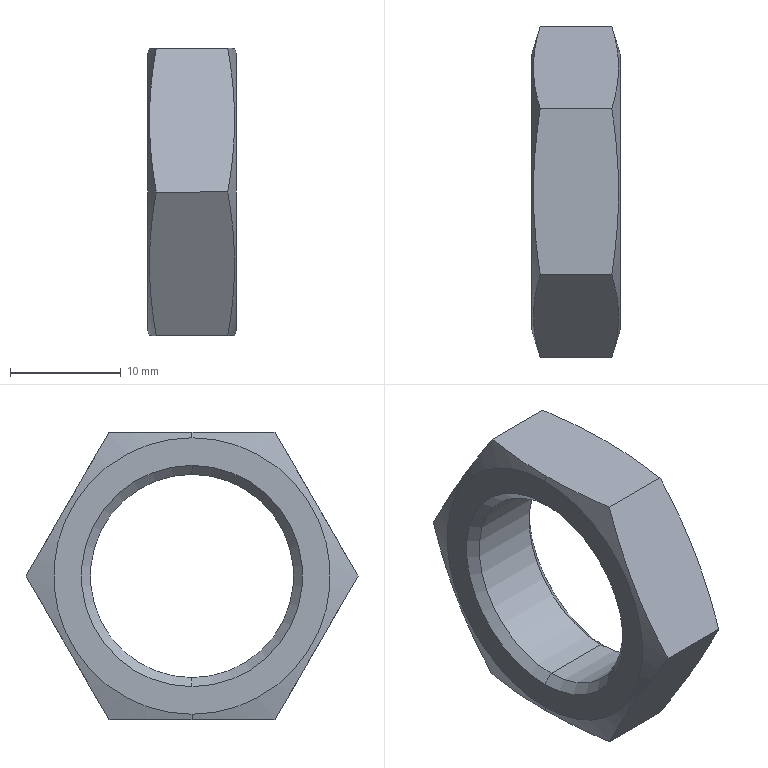Part | SolidWorks | features BaseBody 1 | 1 solid | 18 faces | box 8 x 30.022 x 26 mm | volume 2480 mm3 | cone 8 | plane 8 | cylinder 2 | commonest cylinder face diameters 18.376 x2
STEP:
#1=CARTESIAN_POINT('',(0.812,0.,9.188));
#2=VERTEX_POINT('',#1);
#3=CARTESIAN_POINT('',(0.812,0.,-9.188));
#4=VERTEX_POINT('',#3);
#5=CARTESIAN_POINT('',(0.812,0.,0.));
#6=DIRECTION('',(1.,0.,0.));
#7=DIRECTION('',(0.,0.,-1.));
#8=AXIS2_PLACEMENT_3D('',#5,#6,#7);
#9=CIRCLE('',#8,9.188);
#10=EDGE_CURVE('',#2,#4,#9,.T.);
#11=ORIENTED_EDGE('',*,*,#10,.F.);
#12=CARTESIAN_POINT('',(7.188,0.,9.188));
#13=VERTEX_POINT('',#12);
#14=CARTESIAN_POINT('',(0.,0.,9.188));
#15=DIRECTION('',(1.,0.,0.));
#16=VECTOR('',#15,1000.);
#17=LINE('',#14,#16);
#18=EDGE_CURVE('',#2,#13,#17,.T.);
#19=ORIENTED_EDGE('',*,*,#18,.T.);
#20=CARTESIAN_POINT('',(7.188,0.,-9.188));
#21=VERTEX_POINT('',#20);
#22=CARTESIAN_POINT('',(7.188,0.,0.));
#23=DIRECTION('',(-1.,0.,0.));
#24=DIRECTION('',(0.,0.,-1.));
#25=AXIS2_PLACEMENT_3D('',#22,#23,#24);
#26=CIRCLE('',#25,9.188);
#27=EDGE_CURVE('',#21,#13,#26,.T.);
#28=ORIENTED_EDGE('',*,*,#27,.F.);
#29=CARTESIAN_POINT('',(0.,0.,-9.188));
#30=DIRECTION('',(1.,0.,0.));
#31=VECTOR('',#30,1000.);
#32=LINE('',#29,#31);
#33=EDGE_CURVE('',#4,#21,#32,.T.);
#34=ORIENTED_EDGE('',*,*,#33,.F.);
#35=EDGE_LOOP('',(#11,#19,#28,#34));
#36=FACE_OUTER_BOUND('',#35,.T.);
#37=CARTESIAN_POINT('',(0.,0.,0.));
#38=DIRECTION('',(1.,0.,0.));
#39=DIRECTION('',(0.,0.,-1.));
#40=AXIS2_PLACEMENT_3D('',#37,#38,#39);
#41=CYLINDRICAL_SURFACE('',#40,9.188);
#42=ADVANCED_FACE('',(#36),#41,.F.);
#43=ORIENTED_EDGE('',*,*,#27,.T.);
#44=CARTESIAN_POINT('',(8.,0.,10.));
#45=VERTEX_POINT('',#44);
#46=CARTESIAN_POINT('',(8.,0.,10.));
#47=DIRECTION('',(0.7071,0.,0.7071));
#48=VECTOR('',#47,1000.);
#49=LINE('',#46,#48);
#50=EDGE_CURVE('',#13,#45,#49,.T.);
#51=ORIENTED_EDGE('',*,*,#50,.T.);
#52=CARTESIAN_POINT('',(8.,0.,-10.));
#53=VERTEX_POINT('',#52);
#54=CARTESIAN_POINT('',(8.,0.,0.));
#55=DIRECTION('',(-1.,0.,0.));
#56=DIRECTION('',(0.,0.,-1.));
#57=AXIS2_PLACEMENT_3D('',#54,#55,#56);
#58=CIRCLE('',#57,10.);
#59=EDGE_CURVE('',#53,#45,#58,.T.);
#60=ORIENTED_EDGE('',*,*,#59,.F.);
#61=CARTESIAN_POINT('',(8.,0.,-10.));
#62=DIRECTION('',(0.7071,0.,-0.7071));
#63=VECTOR('',#62,1000.);
#64=LINE('',#61,#63);
#65=EDGE_CURVE('',#21,#53,#64,.T.);
#66=ORIENTED_EDGE('',*,*,#65,.F.);
#67=EDGE_LOOP('',(#43,#51,#60,#66));
#68=FACE_OUTER_BOUND('',#67,.T.);
#69=CARTESIAN_POINT('',(8.,0.,0.));
#70=DIRECTION('',(1.,0.,0.));
#71=DIRECTION('',(0.,0.,-1.));
#72=AXIS2_PLACEMENT_3D('',#69,#70,#71);
#73=CONICAL_SURFACE('',#72,10.,0.7854);
#74=ADVANCED_FACE('',(#68),#73,.F.);
#75=ORIENTED_EDGE('',*,*,#10,.T.);
#76=CARTESIAN_POINT('',(0.,0.,-10.));
#77=VERTEX_POINT('',#76);
#78=CARTESIAN_POINT('',(0.,0.,-10.));
#79=DIRECTION('',(-0.7071,0.,-0.7071));
#80=VECTOR('',#79,1000.);
#81=LINE('',#78,#80);
#82=EDGE_CURVE('',#4,#77,#81,.T.);
#83=ORIENTED_EDGE('',*,*,#82,.T.);
#84=CARTESIAN_POINT('',(0.,0.,10.));
#85=VERTEX_POINT('',#84);
#86=CARTESIAN_POINT('',(0.,0.,0.));
#87=DIRECTION('',(1.,0.,0.));
#88=DIRECTION('',(0.,0.,1.));
#89=AXIS2_PLACEMENT_3D('',#86,#87,#88);
#90=CIRCLE('',#89,10.);
#91=EDGE_CURVE('',#85,#77,#90,.T.);
#92=ORIENTED_EDGE('',*,*,#91,.F.);
#93=CARTESIAN_POINT('',(0.,0.,10.));
#94=DIRECTION('',(-0.7071,0.,0.7071));
#95=VECTOR('',#94,1000.);
#96=LINE('',#93,#95);
#97=EDGE_CURVE('',#2,#85,#96,.T.);
#98=ORIENTED_EDGE('',*,*,#97,.F.);
#99=EDGE_LOOP('',(#75,#83,#92,#98));
#100=FACE_OUTER_BOUND('',#99,.T.);
#101=CARTESIAN_POINT('',(0.,0.,0.));
#102=DIRECTION('',(-1.,0.,0.));
#103=DIRECTION('',(0.,0.,1.));
#104=AXIS2_PLACEMENT_3D('',#101,#102,#103);
#105=CONICAL_SURFACE('',#104,10.,0.7854);
#106=ADVANCED_FACE('',(#100),#105,.F.);
#107=CARTESIAN_POINT('',(8.,0.,-12.5));
#108=VERTEX_POINT('',#107);
#109=CARTESIAN_POINT('',(8.,0.,12.5));
#110=VERTEX_POINT('',#109);
#111=CARTESIAN_POINT('',(8.,0.,0.));
#112=DIRECTION('',(1.,0.,0.));
#113=DIRECTION('',(0.,0.,1.));
#114=AXIS2_PLACEMENT_3D('',#111,#112,#113);
#115=CIRCLE('',#114,12.5);
#116=EDGE_CURVE('',#108,#110,#115,.T.);
#117=ORIENTED_EDGE('',*,*,#116,.F.);
#118=CARTESIAN_POINT('',(7.848,0.,-13.));
#119=VERTEX_POINT('',#118);
#120=CARTESIAN_POINT('',(7.231,0.,-15.026));
#121=DIRECTION('',(-0.2912,0.,-0.9567));
#122=VECTOR('',#121,1000.);
#123=LINE('',#120,#122);
#124=EDGE_CURVE('',#108,#119,#123,.T.);
#125=ORIENTED_EDGE('',*,*,#124,.T.);
#126=CARTESIAN_POINT('',(7.236,7.506,-13.));
#127=VERTEX_POINT('',#126);
#128=CARTESIAN_POINT('',(7.848,0.,-13.));
#129=CARTESIAN_POINT('',(7.848,1.251,-13.));
#130=CARTESIAN_POINT('',(7.792,2.502,-13.));
#131=CARTESIAN_POINT('',(7.581,5.004,-13.));
#132=CARTESIAN_POINT('',(7.426,6.255,-13.));
#133=CARTESIAN_POINT('',(7.236,7.506,-13.));
#134=B_SPLINE_CURVE_WITH_KNOTS('',3,(#128,#129,#130,#131,#132,#133),.UNSPECIFIED.,.F.,.F.,(4,2,4),(0.007506,0.01126,0.01501),.UNSPECIFIED.);
#135=EDGE_CURVE('',#119,#127,#134,.T.);
#136=ORIENTED_EDGE('',*,*,#135,.T.);
#137=CARTESIAN_POINT('',(7.236,15.011,-0.000000041));
#138=VERTEX_POINT('',#137);
#139=CARTESIAN_POINT('',(7.236,7.506,-13.));
#140=CARTESIAN_POINT('',(7.426,8.131,-11.917));
#141=CARTESIAN_POINT('',(7.581,8.756,-10.833));
#142=CARTESIAN_POINT('',(7.792,10.007,-8.667));
#143=CARTESIAN_POINT('',(7.904,11.258,-6.5));
#144=CARTESIAN_POINT('',(7.792,12.509,-4.333));
#145=CARTESIAN_POINT('',(7.581,13.76,-2.167));
#146=CARTESIAN_POINT('',(7.426,14.386,-1.083));
#147=CARTESIAN_POINT('',(7.236,15.011,-0.000000041));
#148=B_SPLINE_CURVE_WITH_KNOTS('',3,(#139,#140,#141,#142,#143,#144,#145,#146,#147),.UNSPECIFIED.,.F.,.F.,(4,2,1,2,4),(0.,0.003753,0.007506,0.01126,0.01501),.UNSPECIFIED.);
#149=EDGE_CURVE('',#127,#138,#148,.T.);
#150=ORIENTED_EDGE('',*,*,#149,.T.);
#151=CARTESIAN_POINT('',(7.236,7.506,13.));
#152=VERTEX_POINT('',#151);
#153=CARTESIAN_POINT('',(7.236,15.011,-0.000000041));
#154=CARTESIAN_POINT('',(7.426,14.386,1.083));
#155=CARTESIAN_POINT('',(7.581,13.76,2.167));
#156=CARTESIAN_POINT('',(7.792,12.509,4.333));
#157=CARTESIAN_POINT('',(7.904,11.258,6.5));
#158=CARTESIAN_POINT('',(7.792,10.007,8.667));
#159=CARTESIAN_POINT('',(7.581,8.756,10.833));
#160=CARTESIAN_POINT('',(7.426,8.131,11.917));
#161=CARTESIAN_POINT('',(7.236,7.506,13.));
#162=B_SPLINE_CURVE_WITH_KNOTS('',3,(#153,#154,#155,#156,#157,#158,#159,#160,#161),.UNSPECIFIED.,.F.,.F.,(4,2,1,2,4),(0.,0.003753,0.007506,0.01126,0.01501),.UNSPECIFIED.);
#163=EDGE_CURVE('',#138,#152,#162,.T.);
#164=ORIENTED_EDGE('',*,*,#163,.T.);
#165=CARTESIAN_POINT('',(7.848,0.,13.));
#166=VERTEX_POINT('',#165);
#167=CARTESIAN_POINT('',(7.236,7.506,13.));
#168=CARTESIAN_POINT('',(7.426,6.255,13.));
#169=CARTESIAN_POINT('',(7.581,5.004,13.));
#170=CARTESIAN_POINT('',(7.792,2.502,13.));
#171=CARTESIAN_POINT('',(7.848,1.251,13.));
#172=CARTESIAN_POINT('',(7.848,0.,13.));
#173=B_SPLINE_CURVE_WITH_KNOTS('',3,(#167,#168,#169,#170,#171,#172),.UNSPECIFIED.,.F.,.F.,(4,2,4),(0.,0.003753,0.007506),.UNSPECIFIED.);
#174=EDGE_CURVE('',#152,#166,#173,.T.);
#175=ORIENTED_EDGE('',*,*,#174,.T.);
#176=CARTESIAN_POINT('',(7.231,0.,15.026));
#177=DIRECTION('',(-0.2912,0.,0.9567));
#178=VECTOR('',#177,1000.);
#179=LINE('',#176,#178);
#180=EDGE_CURVE('',#110,#166,#179,.T.);
#181=ORIENTED_EDGE('',*,*,#180,.F.);
#182=EDGE_LOOP('',(#117,#125,#136,#150,#164,#175,#181));
#183=FACE_OUTER_BOUND('',#182,.T.);
#184=CARTESIAN_POINT('',(7.231,0.,0.));
#185=DIRECTION('',(-1.,0.,0.));
#186=DIRECTION('',(0.,0.,1.));
#187=AXIS2_PLACEMENT_3D('',#184,#185,#186);
#188=CONICAL_SURFACE('',#187,15.026,1.275);
#189=ADVANCED_FACE('',(#183),#188,.T.);
#190=CARTESIAN_POINT('',(0.,0.,12.5));
#191=VERTEX_POINT('',#190);
#192=CARTESIAN_POINT('',(0.,0.,-12.5));
#193=VERTEX_POINT('',#192);
#194=CARTESIAN_POINT('',(0.,0.,0.));
#195=DIRECTION('',(-1.,0.,0.));
#196=DIRECTION('',(0.,0.,-1.));
#197=AXIS2_PLACEMENT_3D('',#194,#195,#196);
#198=CIRCLE('',#197,12.5);
#199=EDGE_CURVE('',#191,#193,#198,.T.);
#200=ORIENTED_EDGE('',*,*,#199,.F.);
#201=CARTESIAN_POINT('',(0.1522,0.,13.));
#202=VERTEX_POINT('',#201);
#203=CARTESIAN_POINT('',(0.7688,0.,15.026));
#204=DIRECTION('',(0.2912,0.,0.9567));
#205=VECTOR('',#204,1000.);
#206=LINE('',#203,#205);
#207=EDGE_CURVE('',#191,#202,#206,.T.);
#208=ORIENTED_EDGE('',*,*,#207,.T.);
#209=CARTESIAN_POINT('',(0.7642,7.506,13.));
#210=VERTEX_POINT('',#209);
#211=CARTESIAN_POINT('',(0.1522,0.,13.));
#212=CARTESIAN_POINT('',(0.1522,1.251,13.));
#213=CARTESIAN_POINT('',(0.2081,2.502,13.));
#214=CARTESIAN_POINT('',(0.4193,5.004,13.));
#215=CARTESIAN_POINT('',(0.5739,6.255,13.));
#216=CARTESIAN_POINT('',(0.7642,7.506,13.));
#217=B_SPLINE_CURVE_WITH_KNOTS('',3,(#211,#212,#213,#214,#215,#216),.UNSPECIFIED.,.F.,.F.,(4,2,4),(0.007506,0.01126,0.01501),.UNSPECIFIED.);
#218=EDGE_CURVE('',#202,#210,#217,.T.);
#219=ORIENTED_EDGE('',*,*,#218,.T.);
#220=CARTESIAN_POINT('',(0.7642,15.011,0.000000041));
#221=VERTEX_POINT('',#220);
#222=CARTESIAN_POINT('',(0.7642,7.506,13.));
#223=CARTESIAN_POINT('',(0.5739,8.131,11.917));
#224=CARTESIAN_POINT('',(0.4193,8.756,10.833));
#225=CARTESIAN_POINT('',(0.2081,10.007,8.667));
#226=CARTESIAN_POINT('',(0.09621,11.258,6.5));
#227=CARTESIAN_POINT('',(0.2081,12.509,4.333));
#228=CARTESIAN_POINT('',(0.4193,13.76,2.167));
#229=CARTESIAN_POINT('',(0.5739,14.386,1.083));
#230=CARTESIAN_POINT('',(0.7642,15.011,0.000000041));
#231=B_SPLINE_CURVE_WITH_KNOTS('',3,(#222,#223,#224,#225,#226,#227,#228,#229,#230),.UNSPECIFIED.,.F.,.F.,(4,2,1,2,4),(0.,0.003753,0.007506,0.01126,0.01501),.UNSPECIFIED.);
#232=EDGE_CURVE('',#210,#221,#231,.T.);
#233=ORIENTED_EDGE('',*,*,#232,.T.);
#234=CARTESIAN_POINT('',(0.7642,7.506,-13.));
#235=VERTEX_POINT('',#234);
#236=CARTESIAN_POINT('',(0.7642,15.011,0.000000041));
#237=CARTESIAN_POINT('',(0.5739,14.386,-1.083));
#238=CARTESIAN_POINT('',(0.4193,13.76,-2.167));
#239=CARTESIAN_POINT('',(0.2081,12.509,-4.333));
#240=CARTESIAN_POINT('',(0.09621,11.258,-6.5));
#241=CARTESIAN_POINT('',(0.2081,10.007,-8.667));
#242=CARTESIAN_POINT('',(0.4193,8.756,-10.833));
#243=CARTESIAN_POINT('',(0.5739,8.131,-11.917));
#244=CARTESIAN_POINT('',(0.7642,7.506,-13.));
#245=B_SPLINE_CURVE_WITH_KNOTS('',3,(#236,#237,#238,#239,#240,#241,#242,#243,#244),.UNSPECIFIED.,.F.,.F.,(4,2,1,2,4),(0.,0.003753,0.007506,0.01126,0.01501),.UNSPECIFIED.);
#246=EDGE_CURVE('',#221,#235,#245,.T.);
#247=ORIENTED_EDGE('',*,*,#246,.T.);
#248=CARTESIAN_POINT('',(0.1522,0.,-13.));
#249=VERTEX_POINT('',#248);
#250=CARTESIAN_POINT('',(0.7642,7.506,-13.));
#251=CARTESIAN_POINT('',(0.5739,6.255,-13.));
#252=CARTESIAN_POINT('',(0.4193,5.004,-13.));
#253=CARTESIAN_POINT('',(0.2081,2.502,-13.));
#254=CARTESIAN_POINT('',(0.1522,1.251,-13.));
#255=CARTESIAN_POINT('',(0.1522,0.,-13.));
#256=B_SPLINE_CURVE_WITH_KNOTS('',3,(#250,#251,#252,#253,#254,#255),.UNSPECIFIED.,.F.,.F.,(4,2,4),(0.,0.003753,0.007506),.UNSPECIFIED.);
#257=EDGE_CURVE('',#235,#249,#256,.T.);
#258=ORIENTED_EDGE('',*,*,#257,.T.);
#259=CARTESIAN_POINT('',(0.7688,0.,-15.026));
#260=DIRECTION('',(0.2912,0.,-0.9567));
#261=VECTOR('',#260,1000.);
#262=LINE('',#259,#261);
#263=EDGE_CURVE('',#193,#249,#262,.T.);
#264=ORIENTED_EDGE('',*,*,#263,.F.);
#265=EDGE_LOOP('',(#200,#208,#219,#233,#247,#258,#264));
#266=FACE_OUTER_BOUND('',#265,.T.);
#267=CARTESIAN_POINT('',(0.7688,0.,0.));
#268=DIRECTION('',(1.,0.,0.));
#269=DIRECTION('',(0.,0.,-1.));
#270=AXIS2_PLACEMENT_3D('',#267,#268,#269);
#271=CONICAL_SURFACE('',#270,15.026,1.275);
#272=ADVANCED_FACE('',(#266),#271,.T.);
#273=ORIENTED_EDGE('',*,*,#18,.F.);
#274=CARTESIAN_POINT('',(0.812,0.,0.));
#275=DIRECTION('',(1.,0.,0.));
#276=DIRECTION('',(0.,0.,-1.));
#277=AXIS2_PLACEMENT_3D('',#274,#275,#276);
#278=CIRCLE('',#277,9.188);
#279=EDGE_CURVE('',#4,#2,#278,.T.);
#280=ORIENTED_EDGE('',*,*,#279,.F.);
#281=ORIENTED_EDGE('',*,*,#33,.T.);
#282=CARTESIAN_POINT('',(7.188,0.,0.));
#283=DIRECTION('',(-1.,0.,0.));
#284=DIRECTION('',(0.,0.,-1.));
#285=AXIS2_PLACEMENT_3D('',#282,#283,#284);
#286=CIRCLE('',#285,9.188);
#287=EDGE_CURVE('',#13,#21,#286,.T.);
#288=ORIENTED_EDGE('',*,*,#287,.F.);
#289=EDGE_LOOP('',(#273,#280,#281,#288));
#290=FACE_OUTER_BOUND('',#289,.T.);
#291=CARTESIAN_POINT('',(0.,0.,0.));
#292=DIRECTION('',(1.,0.,0.));
#293=DIRECTION('',(0.,0.,-1.));
#294=AXIS2_PLACEMENT_3D('',#291,#292,#293);
#295=CYLINDRICAL_SURFACE('',#294,9.188);
#296=ADVANCED_FACE('',(#290),#295,.F.);
#297=ORIENTED_EDGE('',*,*,#50,.F.);
#298=ORIENTED_EDGE('',*,*,#287,.T.);
#299=ORIENTED_EDGE('',*,*,#65,.T.);
#300=CARTESIAN_POINT('',(8.,0.,0.));
#301=DIRECTION('',(-1.,0.,0.));
#302=DIRECTION('',(0.,0.,-1.));
#303=AXIS2_PLACEMENT_3D('',#300,#301,#302);
#304=CIRCLE('',#303,10.);
#305=EDGE_CURVE('',#45,#53,#304,.T.);
#306=ORIENTED_EDGE('',*,*,#305,.F.);
#307=EDGE_LOOP('',(#297,#298,#299,#306));
#308=FACE_OUTER_BOUND('',#307,.T.);
#309=CARTESIAN_POINT('',(8.,0.,0.));
#310=DIRECTION('',(1.,0.,0.));
#311=DIRECTION('',(0.,0.,-1.));
#312=AXIS2_PLACEMENT_3D('',#309,#310,#311);
#313=CONICAL_SURFACE('',#312,10.,0.7854);
#314=ADVANCED_FACE('',(#308),#313,.F.);
#315=ORIENTED_EDGE('',*,*,#82,.F.);
#316=ORIENTED_EDGE('',*,*,#279,.T.);
#317=ORIENTED_EDGE('',*,*,#97,.T.);
#318=CARTESIAN_POINT('',(0.,0.,0.));
#319=DIRECTION('',(1.,0.,0.));
#320=DIRECTION('',(0.,0.,1.));
#321=AXIS2_PLACEMENT_3D('',#318,#319,#320);
#322=CIRCLE('',#321,10.);
#323=EDGE_CURVE('',#77,#85,#322,.T.);
#324=ORIENTED_EDGE('',*,*,#323,.F.);
#325=EDGE_LOOP('',(#315,#316,#317,#324));
#326=FACE_OUTER_BOUND('',#325,.T.);
#327=CARTESIAN_POINT('',(0.,0.,0.));
#328=DIRECTION('',(-1.,0.,0.));
#329=DIRECTION('',(0.,0.,1.));
#330=AXIS2_PLACEMENT_3D('',#327,#328,#329);
#331=CONICAL_SURFACE('',#330,10.,0.7854);
#332=ADVANCED_FACE('',(#326),#331,.F.);
#333=CARTESIAN_POINT('',(8.,0.,0.));
#334=DIRECTION('',(1.,0.,0.));
#335=DIRECTION('',(0.,0.,1.));
#336=AXIS2_PLACEMENT_3D('',#333,#334,#335);
#337=CIRCLE('',#336,12.5);
#338=EDGE_CURVE('',#110,#108,#337,.T.);
#339=ORIENTED_EDGE('',*,*,#338,.T.);
#340=ORIENTED_EDGE('',*,*,#116,.T.);
#341=EDGE_LOOP('',(#339,#340));
#342=FACE_OUTER_BOUND('',#341,.T.);
#343=ORIENTED_EDGE('',*,*,#59,.T.);
#344=ORIENTED_EDGE('',*,*,#305,.T.);
#345=EDGE_LOOP('',(#343,#344));
#346=FACE_BOUND('',#345,.T.);
#347=CARTESIAN_POINT('',(8.,-12.5,0.));
#348=DIRECTION('',(1.,0.,0.));
#349=DIRECTION('',(0.,0.,-1.));
#350=AXIS2_PLACEMENT_3D('',#347,#348,#349);
#351=PLANE('',#350);
#352=ADVANCED_FACE('',(#342,#346),#351,.T.);
#353=ORIENTED_EDGE('',*,*,#91,.T.);
#354=ORIENTED_EDGE('',*,*,#323,.T.);
#355=EDGE_LOOP('',(#353,#354));
#356=FACE_BOUND('',#355,.T.);
#357=CARTESIAN_POINT('',(0.,0.,0.));
#358=DIRECTION('',(-1.,0.,0.));
#359=DIRECTION('',(0.,0.,-1.));
#360=AXIS2_PLACEMENT_3D('',#357,#358,#359);
#361=CIRCLE('',#360,12.5);
#362=EDGE_CURVE('',#193,#191,#361,.T.);
#363=ORIENTED_EDGE('',*,*,#362,.T.);
#364=ORIENTED_EDGE('',*,*,#199,.T.);
#365=EDGE_LOOP('',(#363,#364));
#366=FACE_OUTER_BOUND('',#365,.T.);
#367=CARTESIAN_POINT('',(0.,-10.,0.));
#368=DIRECTION('',(-1.,0.,0.));
#369=DIRECTION('',(0.,0.,1.));
#370=AXIS2_PLACEMENT_3D('',#367,#368,#369);
#371=PLANE('',#370);
#372=ADVANCED_FACE('',(#356,#366),#371,.T.);
#373=ORIENTED_EDGE('',*,*,#124,.F.);
#374=ORIENTED_EDGE('',*,*,#338,.F.);
#375=ORIENTED_EDGE('',*,*,#180,.T.);
#376=CARTESIAN_POINT('',(7.236,-7.506,13.));
#377=VERTEX_POINT('',#376);
#378=CARTESIAN_POINT('',(7.848,0.,13.));
#379=CARTESIAN_POINT('',(7.848,-1.251,13.));
#380=CARTESIAN_POINT('',(7.792,-2.502,13.));
#381=CARTESIAN_POINT('',(7.581,-5.004,13.));
#382=CARTESIAN_POINT('',(7.426,-6.255,13.));
#383=CARTESIAN_POINT('',(7.236,-7.506,13.));
#384=B_SPLINE_CURVE_WITH_KNOTS('',3,(#378,#379,#380,#381,#382,#383),.UNSPECIFIED.,.F.,.F.,(4,2,4),(0.007506,0.01126,0.01501),.UNSPECIFIED.);
#385=EDGE_CURVE('',#166,#377,#384,.T.);
#386=ORIENTED_EDGE('',*,*,#385,.T.);
#387=CARTESIAN_POINT('',(7.236,-15.011,0.000000041));
#388=VERTEX_POINT('',#387);
#389=CARTESIAN_POINT('',(7.236,-7.506,13.));
#390=CARTESIAN_POINT('',(7.426,-8.131,11.917));
#391=CARTESIAN_POINT('',(7.581,-8.756,10.833));
#392=CARTESIAN_POINT('',(7.792,-10.007,8.667));
#393=CARTESIAN_POINT('',(7.904,-11.258,6.5));
#394=CARTESIAN_POINT('',(7.792,-12.509,4.333));
#395=CARTESIAN_POINT('',(7.581,-13.76,2.167));
#396=CARTESIAN_POINT('',(7.426,-14.386,1.083));
#397=CARTESIAN_POINT('',(7.236,-15.011,0.000000041));
#398=B_SPLINE_CURVE_WITH_KNOTS('',3,(#389,#390,#391,#392,#393,#394,#395,#396,#397),.UNSPECIFIED.,.F.,.F.,(4,2,1,2,4),(0.,0.003753,0.007506,0.01126,0.01501),.UNSPECIFIED.);
#399=EDGE_CURVE('',#377,#388,#398,.T.);
#400=ORIENTED_EDGE('',*,*,#399,.T.);
#401=CARTESIAN_POINT('',(7.236,-7.506,-13.));
#402=VERTEX_POINT('',#401);
#403=CARTESIAN_POINT('',(7.236,-15.011,0.000000041));
#404=CARTESIAN_POINT('',(7.426,-14.386,-1.083));
#405=CARTESIAN_POINT('',(7.581,-13.76,-2.167));
#406=CARTESIAN_POINT('',(7.792,-12.509,-4.333));
#407=CARTESIAN_POINT('',(7.904,-11.258,-6.5));
#408=CARTESIAN_POINT('',(7.792,-10.007,-8.667));
#409=CARTESIAN_POINT('',(7.581,-8.756,-10.833));
#410=CARTESIAN_POINT('',(7.426,-8.131,-11.917));
#411=CARTESIAN_POINT('',(7.236,-7.506,-13.));
#412=B_SPLINE_CURVE_WITH_KNOTS('',3,(#403,#404,#405,#406,#407,#408,#409,#410,#411),.UNSPECIFIED.,.F.,.F.,(4,2,1,2,4),(0.,0.003753,0.007506,0.01126,0.01501),.UNSPECIFIED.);
#413=EDGE_CURVE('',#388,#402,#412,.T.);
#414=ORIENTED_EDGE('',*,*,#413,.T.);
#415=CARTESIAN_POINT('',(7.236,-7.506,-13.));
#416=CARTESIAN_POINT('',(7.426,-6.255,-13.));
#417=CARTESIAN_POINT('',(7.581,-5.004,-13.));
#418=CARTESIAN_POINT('',(7.792,-2.502,-13.));
#419=CARTESIAN_POINT('',(7.848,-1.251,-13.));
#420=CARTESIAN_POINT('',(7.848,0.,-13.));
#421=B_SPLINE_CURVE_WITH_KNOTS('',3,(#415,#416,#417,#418,#419,#420),.UNSPECIFIED.,.F.,.F.,(4,2,4),(0.,0.003753,0.007506),.UNSPECIFIED.);
#422=EDGE_CURVE('',#402,#119,#421,.T.);
#423=ORIENTED_EDGE('',*,*,#422,.T.);
#424=EDGE_LOOP('',(#373,#374,#375,#386,#400,#414,#423));
#425=FACE_OUTER_BOUND('',#424,.T.);
#426=CARTESIAN_POINT('',(7.231,0.,0.));
#427=DIRECTION('',(-1.,0.,0.));
#428=DIRECTION('',(0.,0.,1.));
#429=AXIS2_PLACEMENT_3D('',#426,#427,#428);
#430=CONICAL_SURFACE('',#429,15.026,1.275);
#431=ADVANCED_FACE('',(#425),#430,.T.);
#432=ORIENTED_EDGE('',*,*,#207,.F.);
#433=ORIENTED_EDGE('',*,*,#362,.F.);
#434=ORIENTED_EDGE('',*,*,#263,.T.);
#435=CARTESIAN_POINT('',(0.7642,-7.506,-13.));
#436=VERTEX_POINT('',#435);
#437=CARTESIAN_POINT('',(0.1522,0.,-13.));
#438=CARTESIAN_POINT('',(0.1522,-1.251,-13.));
#439=CARTESIAN_POINT('',(0.2081,-2.502,-13.));
#440=CARTESIAN_POINT('',(0.4193,-5.004,-13.));
#441=CARTESIAN_POINT('',(0.5739,-6.255,-13.));
#442=CARTESIAN_POINT('',(0.7642,-7.506,-13.));
#443=B_SPLINE_CURVE_WITH_KNOTS('',3,(#437,#438,#439,#440,#441,#442),.UNSPECIFIED.,.F.,.F.,(4,2,4),(0.007506,0.01126,0.01501),.UNSPECIFIED.);
#444=EDGE_CURVE('',#249,#436,#443,.T.);
#445=ORIENTED_EDGE('',*,*,#444,.T.);
#446=CARTESIAN_POINT('',(0.7642,-15.011,-0.000000041));
#447=VERTEX_POINT('',#446);
#448=CARTESIAN_POINT('',(0.7642,-7.506,-13.));
#449=CARTESIAN_POINT('',(0.5739,-8.131,-11.917));
#450=CARTESIAN_POINT('',(0.4193,-8.756,-10.833));
#451=CARTESIAN_POINT('',(0.2081,-10.007,-8.667));
#452=CARTESIAN_POINT('',(0.09621,-11.258,-6.5));
#453=CARTESIAN_POINT('',(0.2081,-12.509,-4.333));
#454=CARTESIAN_POINT('',(0.4193,-13.76,-2.167));
#455=CARTESIAN_POINT('',(0.5739,-14.386,-1.083));
#456=CARTESIAN_POINT('',(0.7642,-15.011,-0.000000041));
#457=B_SPLINE_CURVE_WITH_KNOTS('',3,(#448,#449,#450,#451,#452,#453,#454,#455,#456),.UNSPECIFIED.,.F.,.F.,(4,2,1,2,4),(0.,0.003753,0.007506,0.01126,0.01501),.UNSPECIFIED.);
#458=EDGE_CURVE('',#436,#447,#457,.T.);
#459=ORIENTED_EDGE('',*,*,#458,.T.);
#460=CARTESIAN_POINT('',(0.7642,-7.506,13.));
#461=VERTEX_POINT('',#460);
#462=CARTESIAN_POINT('',(0.7642,-15.011,-0.000000041));
#463=CARTESIAN_POINT('',(0.5739,-14.386,1.083));
#464=CARTESIAN_POINT('',(0.4193,-13.76,2.167));
#465=CARTESIAN_POINT('',(0.2081,-12.509,4.333));
#466=CARTESIAN_POINT('',(0.09621,-11.258,6.5));
#467=CARTESIAN_POINT('',(0.2081,-10.007,8.667));
#468=CARTESIAN_POINT('',(0.4193,-8.756,10.833));
#469=CARTESIAN_POINT('',(0.5739,-8.131,11.917));
#470=CARTESIAN_POINT('',(0.7642,-7.506,13.));
#471=B_SPLINE_CURVE_WITH_KNOTS('',3,(#462,#463,#464,#465,#466,#467,#468,#469,#470),.UNSPECIFIED.,.F.,.F.,(4,2,1,2,4),(0.,0.003753,0.007506,0.01126,0.01501),.UNSPECIFIED.);
#472=EDGE_CURVE('',#447,#461,#471,.T.);
#473=ORIENTED_EDGE('',*,*,#472,.T.);
#474=CARTESIAN_POINT('',(0.7642,-7.506,13.));
#475=CARTESIAN_POINT('',(0.5739,-6.255,13.));
#476=CARTESIAN_POINT('',(0.4193,-5.004,13.));
#477=CARTESIAN_POINT('',(0.2081,-2.502,13.));
#478=CARTESIAN_POINT('',(0.1522,-1.251,13.));
#479=CARTESIAN_POINT('',(0.1522,0.,13.));
#480=B_SPLINE_CURVE_WITH_KNOTS('',3,(#474,#475,#476,#477,#478,#479),.UNSPECIFIED.,.F.,.F.,(4,2,4),(0.,0.003753,0.007506),.UNSPECIFIED.);
#481=EDGE_CURVE('',#461,#202,#480,.T.);
#482=ORIENTED_EDGE('',*,*,#481,.T.);
#483=EDGE_LOOP('',(#432,#433,#434,#445,#459,#473,#482));
#484=FACE_OUTER_BOUND('',#483,.T.);
#485=CARTESIAN_POINT('',(0.7688,0.,0.));
#486=DIRECTION('',(1.,0.,0.));
#487=DIRECTION('',(0.,0.,-1.));
#488=AXIS2_PLACEMENT_3D('',#485,#486,#487);
#489=CONICAL_SURFACE('',#488,15.026,1.275);
#490=ADVANCED_FACE('',(#484),#489,.T.);
#491=CARTESIAN_POINT('',(8.,7.506,13.));
#492=DIRECTION('',(-1.,0.,0.));
#493=VECTOR('',#492,1000.);
#494=LINE('',#491,#493);
#495=EDGE_CURVE('',#152,#210,#494,.T.);
#496=ORIENTED_EDGE('',*,*,#495,.F.);
#497=ORIENTED_EDGE('',*,*,#163,.F.);
#498=CARTESIAN_POINT('',(8.,15.011,0.));
#499=DIRECTION('',(1.,0.,0.));
#500=VECTOR('',#499,1000.);
#501=LINE('',#498,#500);
#502=EDGE_CURVE('',#221,#138,#501,.T.);
#503=ORIENTED_EDGE('',*,*,#502,.F.);
#504=ORIENTED_EDGE('',*,*,#232,.F.);
#505=EDGE_LOOP('',(#496,#497,#503,#504));
#506=FACE_OUTER_BOUND('',#505,.T.);
#507=CARTESIAN_POINT('',(8.,15.011,0.));
#508=DIRECTION('',(0.,-0.866,-0.5));
#509=DIRECTION('',(0.,0.5,-0.866));
#510=AXIS2_PLACEMENT_3D('',#507,#508,#509);
#511=PLANE('',#510);
#512=ADVANCED_FACE('',(#506),#511,.F.);
#513=ORIENTED_EDGE('',*,*,#502,.T.);
#514=ORIENTED_EDGE('',*,*,#149,.F.);
#515=CARTESIAN_POINT('',(8.,7.506,-13.));
#516=DIRECTION('',(1.,0.,0.));
#517=VECTOR('',#516,1000.);
#518=LINE('',#515,#517);
#519=EDGE_CURVE('',#235,#127,#518,.T.);
#520=ORIENTED_EDGE('',*,*,#519,.F.);
#521=ORIENTED_EDGE('',*,*,#246,.F.);
#522=EDGE_LOOP('',(#513,#514,#520,#521));
#523=FACE_OUTER_BOUND('',#522,.T.);
#524=CARTESIAN_POINT('',(8.,7.506,-13.));
#525=DIRECTION('',(0.,-0.866,0.5));
#526=DIRECTION('',(0.,-0.5,-0.866));
#527=AXIS2_PLACEMENT_3D('',#524,#525,#526);
#528=PLANE('',#527);
#529=ADVANCED_FACE('',(#523),#528,.F.);
#530=ORIENTED_EDGE('',*,*,#519,.T.);
#531=ORIENTED_EDGE('',*,*,#135,.F.);
#532=ORIENTED_EDGE('',*,*,#422,.F.);
#533=CARTESIAN_POINT('',(8.,-7.506,-13.));
#534=DIRECTION('',(1.,0.,0.));
#535=VECTOR('',#534,1000.);
#536=LINE('',#533,#535);
#537=EDGE_CURVE('',#436,#402,#536,.T.);
#538=ORIENTED_EDGE('',*,*,#537,.F.);
#539=ORIENTED_EDGE('',*,*,#444,.F.);
#540=ORIENTED_EDGE('',*,*,#257,.F.);
#541=EDGE_LOOP('',(#530,#531,#532,#538,#539,#540));
#542=FACE_OUTER_BOUND('',#541,.T.);
#543=CARTESIAN_POINT('',(8.,-7.506,-13.));
#544=DIRECTION('',(0.,0.,1.));
#545=DIRECTION('',(1.,0.,0.));
#546=AXIS2_PLACEMENT_3D('',#543,#544,#545);
#547=PLANE('',#546);
#548=ADVANCED_FACE('',(#542),#547,.F.);
#549=ORIENTED_EDGE('',*,*,#537,.T.);
#550=ORIENTED_EDGE('',*,*,#413,.F.);
#551=CARTESIAN_POINT('',(8.,-15.011,0.));
#552=DIRECTION('',(1.,0.,0.));
#553=VECTOR('',#552,1000.);
#554=LINE('',#551,#553);
#555=EDGE_CURVE('',#447,#388,#554,.T.);
#556=ORIENTED_EDGE('',*,*,#555,.F.);
#557=ORIENTED_EDGE('',*,*,#458,.F.);
#558=EDGE_LOOP('',(#549,#550,#556,#557));
#559=FACE_OUTER_BOUND('',#558,.T.);
#560=CARTESIAN_POINT('',(8.,-15.011,0.));
#561=DIRECTION('',(0.,0.866,0.5));
#562=DIRECTION('',(0.,-0.5,0.866));
#563=AXIS2_PLACEMENT_3D('',#560,#561,#562);
#564=PLANE('',#563);
#565=ADVANCED_FACE('',(#559),#564,.F.);
#566=ORIENTED_EDGE('',*,*,#555,.T.);
#567=ORIENTED_EDGE('',*,*,#399,.F.);
#568=CARTESIAN_POINT('',(8.,-7.506,13.));
#569=DIRECTION('',(1.,0.,0.));
#570=VECTOR('',#569,1000.);
#571=LINE('',#568,#570);
#572=EDGE_CURVE('',#461,#377,#571,.T.);
#573=ORIENTED_EDGE('',*,*,#572,.F.);
#574=ORIENTED_EDGE('',*,*,#472,.F.);
#575=EDGE_LOOP('',(#566,#567,#573,#574));
#576=FACE_OUTER_BOUND('',#575,.T.);
#577=CARTESIAN_POINT('',(8.,-7.506,13.));
#578=DIRECTION('',(0.,0.866,-0.5));
#579=DIRECTION('',(0.,0.5,0.866));
#580=AXIS2_PLACEMENT_3D('',#577,#578,#579);
#581=PLANE('',#580);
#582=ADVANCED_FACE('',(#576),#581,.F.);
#583=ORIENTED_EDGE('',*,*,#572,.T.);
#584=ORIENTED_EDGE('',*,*,#385,.F.);
#585=ORIENTED_EDGE('',*,*,#174,.F.);
#586=ORIENTED_EDGE('',*,*,#495,.T.);
#587=ORIENTED_EDGE('',*,*,#218,.F.);
#588=ORIENTED_EDGE('',*,*,#481,.F.);
#589=EDGE_LOOP('',(#583,#584,#585,#586,#587,#588));
#590=FACE_OUTER_BOUND('',#589,.T.);
#591=CARTESIAN_POINT('',(8.,7.506,13.));
#592=DIRECTION('',(0.,0.,-1.));
#593=DIRECTION('',(-1.,0.,0.));
#594=AXIS2_PLACEMENT_3D('',#591,#592,#593);
#595=PLANE('',#594);
#596=ADVANCED_FACE('',(#590),#595,.F.);
#597=CLOSED_SHELL('',(#42,#74,#106,#189,#272,#296,#314,#332,#352,#372,#431,#490,#512,#529,#548,#565,#582,#596));
#598=MANIFOLD_SOLID_BREP('',#597);
#599=CARTESIAN_POINT('',(0.,0.,0.));
#600=DIRECTION('',(0.,0.,1.));
#601=DIRECTION('',(1.,0.,0.));
#602=AXIS2_PLACEMENT_3D('',#599,#600,#601);
#603=(LENGTH_UNIT()NAMED_UNIT(*)SI_UNIT(.MILLI.,.METRE.));
#604=UNCERTAINTY_MEASURE_WITH_UNIT(LENGTH_MEASURE(0.00001),#603,'','');
#605=(NAMED_UNIT(*)PLANE_ANGLE_UNIT()SI_UNIT($,.RADIAN.));
#606=(NAMED_UNIT(*)SI_UNIT($,.STERADIAN.)SOLID_ANGLE_UNIT());
#607=(GEOMETRIC_REPRESENTATION_CONTEXT(3)GLOBAL_UNCERTAINTY_ASSIGNED_CONTEXT((#604))GLOBAL_UNIT_ASSIGNED_CONTEXT((#603,#605,#606))REPRESENTATION_CONTEXT('',''));
#608=ADVANCED_BREP_SHAPE_REPRESENTATION('',(#598,#602),#607);